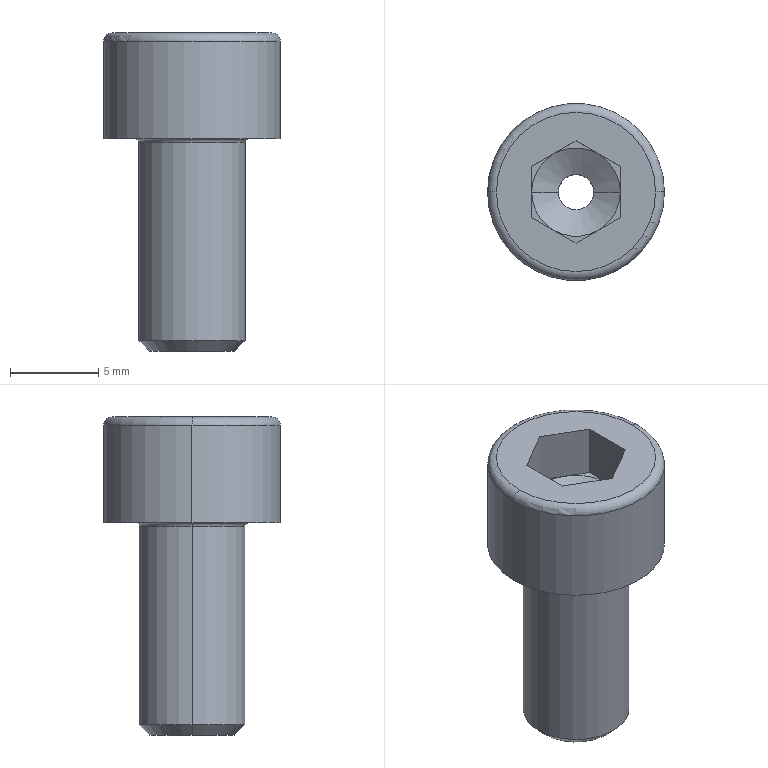Part | SolidWorks | features Fillet 2, ICE 2, Chamfer 1, Revolution 1 | 1 solid | 29 faces | box 10 x 10 x 18 mm | volume 687.683 mm3 | plane 15 | cylinder 6 | torus 4 | cone 4 | commonest cylinder face diameters 2 x2 6 x2 10 x2
STEP:
#1=CARTESIAN_POINT('',(-3.2,0.,0.));
#2=VERTEX_POINT('',#1);
#3=CARTESIAN_POINT('',(3.2,0.,0.));
#4=VERTEX_POINT('',#3);
#5=CARTESIAN_POINT('',(0.,0.,0.));
#6=DIRECTION('',(0.,0.,1.));
#7=DIRECTION('',(1.,0.,0.));
#8=AXIS2_PLACEMENT_3D('',#5,#6,#7);
#9=CIRCLE('',#8,3.2);
#10=EDGE_CURVE('',#2,#4,#9,.T.);
#11=ORIENTED_EDGE('',*,*,#10,.F.);
#12=CARTESIAN_POINT('',(-3.,0.,-0.2));
#13=VERTEX_POINT('',#12);
#14=CARTESIAN_POINT('',(-3.2,0.,-0.2));
#15=DIRECTION('',(0.,1.,0.));
#16=DIRECTION('',(-1.,0.,0.));
#17=AXIS2_PLACEMENT_3D('',#14,#15,#16);
#18=CIRCLE('',#17,0.2);
#19=EDGE_CURVE('',#2,#13,#18,.T.);
#20=ORIENTED_EDGE('',*,*,#19,.T.);
#21=CARTESIAN_POINT('',(3.,0.,-0.2));
#22=VERTEX_POINT('',#21);
#23=CARTESIAN_POINT('',(0.,0.,-0.2));
#24=DIRECTION('',(0.,0.,-1.));
#25=DIRECTION('',(1.,0.,0.));
#26=AXIS2_PLACEMENT_3D('',#23,#24,#25);
#27=CIRCLE('',#26,3.);
#28=EDGE_CURVE('',#22,#13,#27,.T.);
#29=ORIENTED_EDGE('',*,*,#28,.F.);
#30=CARTESIAN_POINT('',(3.2,0.,-0.2));
#31=DIRECTION('',(0.,-1.,0.));
#32=DIRECTION('',(0.,0.,-1.));
#33=AXIS2_PLACEMENT_3D('',#30,#31,#32);
#34=CIRCLE('',#33,0.2);
#35=EDGE_CURVE('',#4,#22,#34,.T.);
#36=ORIENTED_EDGE('',*,*,#35,.F.);
#37=EDGE_LOOP('',(#11,#20,#29,#36));
#38=FACE_OUTER_BOUND('',#37,.T.);
#39=CARTESIAN_POINT('',(0.,0.,-0.2));
#40=DIRECTION('',(0.,0.,1.));
#41=DIRECTION('',(1.,0.,0.));
#42=AXIS2_PLACEMENT_3D('',#39,#40,#41);
#43=TOROIDAL_SURFACE('',#42,3.2,0.2);
#44=ADVANCED_FACE('',(#38),#43,.F.);
#45=CARTESIAN_POINT('',(-1.,0.,2.134));
#46=VERTEX_POINT('',#45);
#47=CARTESIAN_POINT('',(1.,0.,2.134));
#48=VERTEX_POINT('',#47);
#49=CARTESIAN_POINT('',(0.,0.,2.134));
#50=DIRECTION('',(0.,0.,1.));
#51=DIRECTION('',(1.,0.,0.));
#52=AXIS2_PLACEMENT_3D('',#49,#50,#51);
#53=CIRCLE('',#52,1.);
#54=EDGE_CURVE('',#46,#48,#53,.T.);
#55=ORIENTED_EDGE('',*,*,#54,.F.);
#56=CARTESIAN_POINT('',(-2.5,0.,3.));
#57=VERTEX_POINT('',#56);
#58=CARTESIAN_POINT('',(-2.5,0.,3.));
#59=DIRECTION('',(-0.866,0.,0.5));
#60=VECTOR('',#59,1000.);
#61=LINE('',#58,#60);
#62=EDGE_CURVE('',#46,#57,#61,.T.);
#63=ORIENTED_EDGE('',*,*,#62,.T.);
#64=CARTESIAN_POINT('',(-1.25,-2.165,3.));
#65=VERTEX_POINT('',#64);
#66=CARTESIAN_POINT('',(0.,0.,3.));
#67=DIRECTION('',(0.,0.,1.));
#68=DIRECTION('',(1.,0.,0.));
#69=AXIS2_PLACEMENT_3D('',#66,#67,#68);
#70=CIRCLE('',#69,2.5);
#71=EDGE_CURVE('',#57,#65,#70,.T.);
#72=ORIENTED_EDGE('',*,*,#71,.T.);
#73=CARTESIAN_POINT('',(1.25,-2.165,3.));
#74=VERTEX_POINT('',#73);
#75=CARTESIAN_POINT('',(0.,0.,3.));
#76=DIRECTION('',(0.,0.,1.));
#77=DIRECTION('',(1.,0.,0.));
#78=AXIS2_PLACEMENT_3D('',#75,#76,#77);
#79=CIRCLE('',#78,2.5);
#80=EDGE_CURVE('',#65,#74,#79,.T.);
#81=ORIENTED_EDGE('',*,*,#80,.T.);
#82=CARTESIAN_POINT('',(2.5,0.,3.));
#83=VERTEX_POINT('',#82);
#84=CARTESIAN_POINT('',(0.,0.,3.));
#85=DIRECTION('',(0.,0.,1.));
#86=DIRECTION('',(1.,0.,0.));
#87=AXIS2_PLACEMENT_3D('',#84,#85,#86);
#88=CIRCLE('',#87,2.5);
#89=EDGE_CURVE('',#74,#83,#88,.T.);
#90=ORIENTED_EDGE('',*,*,#89,.T.);
#91=CARTESIAN_POINT('',(2.5,0.,3.));
#92=DIRECTION('',(0.866,0.,0.5));
#93=VECTOR('',#92,1000.);
#94=LINE('',#91,#93);
#95=EDGE_CURVE('',#48,#83,#94,.T.);
#96=ORIENTED_EDGE('',*,*,#95,.F.);
#97=EDGE_LOOP('',(#55,#63,#72,#81,#90,#96));
#98=FACE_OUTER_BOUND('',#97,.T.);
#99=CARTESIAN_POINT('',(0.,0.,3.));
#100=DIRECTION('',(0.,0.,1.));
#101=DIRECTION('',(1.,0.,0.));
#102=AXIS2_PLACEMENT_3D('',#99,#100,#101);
#103=CONICAL_SURFACE('',#102,2.5,1.047);
#104=ADVANCED_FACE('',(#98),#103,.F.);
#105=CARTESIAN_POINT('',(-2.4,0.,-12.));
#106=VERTEX_POINT('',#105);
#107=CARTESIAN_POINT('',(2.4,0.,-12.));
#108=VERTEX_POINT('',#107);
#109=CARTESIAN_POINT('',(0.,0.,-12.));
#110=DIRECTION('',(0.,0.,-1.));
#111=DIRECTION('',(1.,0.,0.));
#112=AXIS2_PLACEMENT_3D('',#109,#110,#111);
#113=CIRCLE('',#112,2.4);
#114=EDGE_CURVE('',#106,#108,#113,.T.);
#115=ORIENTED_EDGE('',*,*,#114,.F.);
#116=CARTESIAN_POINT('',(-3.,0.,-11.4));
#117=VERTEX_POINT('',#116);
#118=CARTESIAN_POINT('',(-3.,0.,-11.4));
#119=DIRECTION('',(-0.7071,0.,0.7071));
#120=VECTOR('',#119,1000.);
#121=LINE('',#118,#120);
#122=EDGE_CURVE('',#106,#117,#121,.T.);
#123=ORIENTED_EDGE('',*,*,#122,.T.);
#124=CARTESIAN_POINT('',(3.,0.,-11.4));
#125=VERTEX_POINT('',#124);
#126=CARTESIAN_POINT('',(0.,0.,-11.4));
#127=DIRECTION('',(0.,0.,1.));
#128=DIRECTION('',(1.,0.,0.));
#129=AXIS2_PLACEMENT_3D('',#126,#127,#128);
#130=CIRCLE('',#129,3.);
#131=EDGE_CURVE('',#125,#117,#130,.T.);
#132=ORIENTED_EDGE('',*,*,#131,.F.);
#133=CARTESIAN_POINT('',(3.,0.,-11.4));
#134=DIRECTION('',(0.7071,0.,0.7071));
#135=VECTOR('',#134,1000.);
#136=LINE('',#133,#135);
#137=EDGE_CURVE('',#108,#125,#136,.T.);
#138=ORIENTED_EDGE('',*,*,#137,.F.);
#139=EDGE_LOOP('',(#115,#123,#132,#138));
#140=FACE_OUTER_BOUND('',#139,.T.);
#141=CARTESIAN_POINT('',(0.,0.,-11.4));
#142=DIRECTION('',(0.,0.,1.));
#143=DIRECTION('',(1.,0.,0.));
#144=AXIS2_PLACEMENT_3D('',#141,#142,#143);
#145=CONICAL_SURFACE('',#144,3.,0.7854);
#146=ADVANCED_FACE('',(#140),#145,.T.);
#147=CARTESIAN_POINT('',(4.5,0.,6.));
#148=VERTEX_POINT('',#147);
#149=CARTESIAN_POINT('',(-4.5,0.,6.));
#150=VERTEX_POINT('',#149);
#151=CARTESIAN_POINT('',(0.,0.,6.));
#152=DIRECTION('',(0.,0.,1.));
#153=DIRECTION('',(-1.,0.,0.));
#154=AXIS2_PLACEMENT_3D('',#151,#152,#153);
#155=CIRCLE('',#154,4.5);
#156=EDGE_CURVE('',#148,#150,#155,.T.);
#157=ORIENTED_EDGE('',*,*,#156,.F.);
#158=CARTESIAN_POINT('',(5.,0.,5.5));
#159=VERTEX_POINT('',#158);
#160=CARTESIAN_POINT('',(4.5,0.,5.5));
#161=DIRECTION('',(0.,1.,0.));
#162=DIRECTION('',(-1.,0.,0.));
#163=AXIS2_PLACEMENT_3D('',#160,#161,#162);
#164=CIRCLE('',#163,0.5);
#165=EDGE_CURVE('',#148,#159,#164,.T.);
#166=ORIENTED_EDGE('',*,*,#165,.T.);
#167=CARTESIAN_POINT('',(-5.,0.,5.5));
#168=VERTEX_POINT('',#167);
#169=CARTESIAN_POINT('',(0.,0.,5.5));
#170=DIRECTION('',(0.,0.,-1.));
#171=DIRECTION('',(-1.,0.,0.));
#172=AXIS2_PLACEMENT_3D('',#169,#170,#171);
#173=CIRCLE('',#172,5.);
#174=EDGE_CURVE('',#168,#159,#173,.T.);
#175=ORIENTED_EDGE('',*,*,#174,.F.);
#176=CARTESIAN_POINT('',(-4.5,0.,5.5));
#177=DIRECTION('',(0.,-1.,0.));
#178=DIRECTION('',(0.,0.,-1.));
#179=AXIS2_PLACEMENT_3D('',#176,#177,#178);
#180=CIRCLE('',#179,0.5);
#181=EDGE_CURVE('',#150,#168,#180,.T.);
#182=ORIENTED_EDGE('',*,*,#181,.F.);
#183=EDGE_LOOP('',(#157,#166,#175,#182));
#184=FACE_OUTER_BOUND('',#183,.T.);
#185=CARTESIAN_POINT('',(0.,0.,5.5));
#186=DIRECTION('',(0.,0.,-1.));
#187=DIRECTION('',(-1.,0.,0.));
#188=AXIS2_PLACEMENT_3D('',#185,#186,#187);
#189=TOROIDAL_SURFACE('',#188,4.5,0.5);
#190=ADVANCED_FACE('',(#184),#189,.T.);
#191=ORIENTED_EDGE('',*,*,#131,.T.);
#192=CARTESIAN_POINT('',(-3.,0.,6.));
#193=DIRECTION('',(0.,0.,1.));
#194=VECTOR('',#193,1000.);
#195=LINE('',#192,#194);
#196=EDGE_CURVE('',#117,#13,#195,.T.);
#197=ORIENTED_EDGE('',*,*,#196,.T.);
#198=CARTESIAN_POINT('',(0.,0.,-0.2));
#199=DIRECTION('',(0.,0.,-1.));
#200=DIRECTION('',(1.,0.,0.));
#201=AXIS2_PLACEMENT_3D('',#198,#199,#200);
#202=CIRCLE('',#201,3.);
#203=EDGE_CURVE('',#13,#22,#202,.T.);
#204=ORIENTED_EDGE('',*,*,#203,.T.);
#205=CARTESIAN_POINT('',(3.,0.,6.));
#206=DIRECTION('',(0.,0.,1.));
#207=VECTOR('',#206,1000.);
#208=LINE('',#205,#207);
#209=EDGE_CURVE('',#125,#22,#208,.T.);
#210=ORIENTED_EDGE('',*,*,#209,.F.);
#211=EDGE_LOOP('',(#191,#197,#204,#210));
#212=FACE_OUTER_BOUND('',#211,.T.);
#213=CARTESIAN_POINT('',(0.,0.,6.));
#214=DIRECTION('',(0.,0.,1.));
#215=DIRECTION('',(1.,0.,0.));
#216=AXIS2_PLACEMENT_3D('',#213,#214,#215);
#217=CYLINDRICAL_SURFACE('',#216,3.);
#218=ADVANCED_FACE('',(#212),#217,.T.);
#219=CARTESIAN_POINT('',(5.,0.,0.));
#220=VERTEX_POINT('',#219);
#221=CARTESIAN_POINT('',(-5.,0.,0.));
#222=VERTEX_POINT('',#221);
#223=CARTESIAN_POINT('',(0.,0.,0.));
#224=DIRECTION('',(0.,0.,1.));
#225=DIRECTION('',(1.,0.,0.));
#226=AXIS2_PLACEMENT_3D('',#223,#224,#225);
#227=CIRCLE('',#226,5.);
#228=EDGE_CURVE('',#220,#222,#227,.T.);
#229=ORIENTED_EDGE('',*,*,#228,.T.);
#230=CARTESIAN_POINT('',(-5.,0.,6.));
#231=DIRECTION('',(0.,0.,1.));
#232=VECTOR('',#231,1000.);
#233=LINE('',#230,#232);
#234=EDGE_CURVE('',#222,#168,#233,.T.);
#235=ORIENTED_EDGE('',*,*,#234,.T.);
#236=ORIENTED_EDGE('',*,*,#174,.T.);
#237=CARTESIAN_POINT('',(5.,0.,6.));
#238=DIRECTION('',(0.,0.,1.));
#239=VECTOR('',#238,1000.);
#240=LINE('',#237,#239);
#241=EDGE_CURVE('',#220,#159,#240,.T.);
#242=ORIENTED_EDGE('',*,*,#241,.F.);
#243=EDGE_LOOP('',(#229,#235,#236,#242));
#244=FACE_OUTER_BOUND('',#243,.T.);
#245=CARTESIAN_POINT('',(0.,0.,6.));
#246=DIRECTION('',(0.,0.,1.));
#247=DIRECTION('',(1.,0.,0.));
#248=AXIS2_PLACEMENT_3D('',#245,#246,#247);
#249=CYLINDRICAL_SURFACE('',#248,5.);
#250=ADVANCED_FACE('',(#244),#249,.T.);
#251=CARTESIAN_POINT('',(-1.,0.,-12.));
#252=VERTEX_POINT('',#251);
#253=CARTESIAN_POINT('',(1.,0.,-12.));
#254=VERTEX_POINT('',#253);
#255=CARTESIAN_POINT('',(0.,0.,-12.));
#256=DIRECTION('',(0.,0.,1.));
#257=DIRECTION('',(1.,0.,0.));
#258=AXIS2_PLACEMENT_3D('',#255,#256,#257);
#259=CIRCLE('',#258,1.);
#260=EDGE_CURVE('',#252,#254,#259,.T.);
#261=ORIENTED_EDGE('',*,*,#260,.F.);
#262=CARTESIAN_POINT('',(-1.,0.,6.));
#263=DIRECTION('',(0.,0.,1.));
#264=VECTOR('',#263,1000.);
#265=LINE('',#262,#264);
#266=EDGE_CURVE('',#252,#46,#265,.T.);
#267=ORIENTED_EDGE('',*,*,#266,.T.);
#268=ORIENTED_EDGE('',*,*,#54,.T.);
#269=CARTESIAN_POINT('',(1.,0.,6.));
#270=DIRECTION('',(0.,0.,1.));
#271=VECTOR('',#270,1000.);
#272=LINE('',#269,#271);
#273=EDGE_CURVE('',#254,#48,#272,.T.);
#274=ORIENTED_EDGE('',*,*,#273,.F.);
#275=EDGE_LOOP('',(#261,#267,#268,#274));
#276=FACE_OUTER_BOUND('',#275,.T.);
#277=CARTESIAN_POINT('',(0.,0.,6.));
#278=DIRECTION('',(0.,0.,1.));
#279=DIRECTION('',(1.,0.,0.));
#280=AXIS2_PLACEMENT_3D('',#277,#278,#279);
#281=CYLINDRICAL_SURFACE('',#280,1.);
#282=ADVANCED_FACE('',(#276),#281,.F.);
#283=CARTESIAN_POINT('',(1.25,2.165,3.));
#284=VERTEX_POINT('',#283);
#285=CARTESIAN_POINT('',(0.,0.,3.));
#286=DIRECTION('',(0.,0.,1.));
#287=DIRECTION('',(1.,0.,0.));
#288=AXIS2_PLACEMENT_3D('',#285,#286,#287);
#289=CIRCLE('',#288,2.5);
#290=EDGE_CURVE('',#83,#284,#289,.T.);
#291=ORIENTED_EDGE('',*,*,#290,.F.);
#292=CARTESIAN_POINT('',(2.5,1.443,3.));
#293=VERTEX_POINT('',#292);
#294=CARTESIAN_POINT('',(2.5,-1.443,3.));
#295=DIRECTION('',(0.,1.,0.));
#296=VECTOR('',#295,1000.);
#297=LINE('',#294,#296);
#298=EDGE_CURVE('',#83,#293,#297,.T.);
#299=ORIENTED_EDGE('',*,*,#298,.T.);
#300=CARTESIAN_POINT('',(2.5,1.443,3.));
#301=DIRECTION('',(-0.866,0.5,0.));
#302=VECTOR('',#301,1000.);
#303=LINE('',#300,#302);
#304=EDGE_CURVE('',#293,#284,#303,.T.);
#305=ORIENTED_EDGE('',*,*,#304,.T.);
#306=EDGE_LOOP('',(#291,#299,#305));
#307=FACE_OUTER_BOUND('',#306,.T.);
#308=CARTESIAN_POINT('',(0.,2.887,3.));
#309=DIRECTION('',(0.,0.,1.));
#310=DIRECTION('',(1.,0.,0.));
#311=AXIS2_PLACEMENT_3D('',#308,#309,#310);
#312=PLANE('',#311);
#313=ADVANCED_FACE('',(#307),#312,.T.);
#314=CARTESIAN_POINT('',(-1.25,2.165,3.));
#315=VERTEX_POINT('',#314);
#316=CARTESIAN_POINT('',(0.,0.,3.));
#317=DIRECTION('',(0.,0.,1.));
#318=DIRECTION('',(1.,0.,0.));
#319=AXIS2_PLACEMENT_3D('',#316,#317,#318);
#320=CIRCLE('',#319,2.5);
#321=EDGE_CURVE('',#284,#315,#320,.T.);
#322=ORIENTED_EDGE('',*,*,#321,.F.);
#323=CARTESIAN_POINT('',(0.,2.887,3.));
#324=VERTEX_POINT('',#323);
#325=CARTESIAN_POINT('',(2.5,1.443,3.));
#326=DIRECTION('',(-0.866,0.5,0.));
#327=VECTOR('',#326,1000.);
#328=LINE('',#325,#327);
#329=EDGE_CURVE('',#284,#324,#328,.T.);
#330=ORIENTED_EDGE('',*,*,#329,.T.);
#331=CARTESIAN_POINT('',(0.,2.887,3.));
#332=DIRECTION('',(-0.866,-0.5,0.));
#333=VECTOR('',#332,1000.);
#334=LINE('',#331,#333);
#335=EDGE_CURVE('',#324,#315,#334,.T.);
#336=ORIENTED_EDGE('',*,*,#335,.T.);
#337=EDGE_LOOP('',(#322,#330,#336));
#338=FACE_OUTER_BOUND('',#337,.T.);
#339=CARTESIAN_POINT('',(0.,2.887,3.));
#340=DIRECTION('',(0.,0.,1.));
#341=DIRECTION('',(1.,0.,0.));
#342=AXIS2_PLACEMENT_3D('',#339,#340,#341);
#343=PLANE('',#342);
#344=ADVANCED_FACE('',(#338),#343,.T.);
#345=CARTESIAN_POINT('',(0.,0.,3.));
#346=DIRECTION('',(0.,0.,1.));
#347=DIRECTION('',(1.,0.,0.));
#348=AXIS2_PLACEMENT_3D('',#345,#346,#347);
#349=CIRCLE('',#348,2.5);
#350=EDGE_CURVE('',#315,#57,#349,.T.);
#351=ORIENTED_EDGE('',*,*,#350,.F.);
#352=CARTESIAN_POINT('',(-2.5,1.443,3.));
#353=VERTEX_POINT('',#352);
#354=CARTESIAN_POINT('',(0.,2.887,3.));
#355=DIRECTION('',(-0.866,-0.5,0.));
#356=VECTOR('',#355,1000.);
#357=LINE('',#354,#356);
#358=EDGE_CURVE('',#315,#353,#357,.T.);
#359=ORIENTED_EDGE('',*,*,#358,.T.);
#360=CARTESIAN_POINT('',(-2.5,1.443,3.));
#361=DIRECTION('',(0.,-1.,0.));
#362=VECTOR('',#361,1000.);
#363=LINE('',#360,#362);
#364=EDGE_CURVE('',#353,#57,#363,.T.);
#365=ORIENTED_EDGE('',*,*,#364,.T.);
#366=EDGE_LOOP('',(#351,#359,#365));
#367=FACE_OUTER_BOUND('',#366,.T.);
#368=CARTESIAN_POINT('',(0.,2.887,3.));
#369=DIRECTION('',(0.,0.,1.));
#370=DIRECTION('',(1.,0.,0.));
#371=AXIS2_PLACEMENT_3D('',#368,#369,#370);
#372=PLANE('',#371);
#373=ADVANCED_FACE('',(#367),#372,.T.);
#374=ORIENTED_EDGE('',*,*,#71,.F.);
#375=CARTESIAN_POINT('',(-2.5,-1.443,3.));
#376=VERTEX_POINT('',#375);
#377=CARTESIAN_POINT('',(-2.5,1.443,3.));
#378=DIRECTION('',(0.,-1.,0.));
#379=VECTOR('',#378,1000.);
#380=LINE('',#377,#379);
#381=EDGE_CURVE('',#57,#376,#380,.T.);
#382=ORIENTED_EDGE('',*,*,#381,.T.);
#383=CARTESIAN_POINT('',(-2.5,-1.443,3.));
#384=DIRECTION('',(0.866,-0.5,0.));
#385=VECTOR('',#384,1000.);
#386=LINE('',#383,#385);
#387=EDGE_CURVE('',#376,#65,#386,.T.);
#388=ORIENTED_EDGE('',*,*,#387,.T.);
#389=EDGE_LOOP('',(#374,#382,#388));
#390=FACE_OUTER_BOUND('',#389,.T.);
#391=CARTESIAN_POINT('',(0.,2.887,3.));
#392=DIRECTION('',(0.,0.,1.));
#393=DIRECTION('',(1.,0.,0.));
#394=AXIS2_PLACEMENT_3D('',#391,#392,#393);
#395=PLANE('',#394);
#396=ADVANCED_FACE('',(#390),#395,.T.);
#397=ORIENTED_EDGE('',*,*,#80,.F.);
#398=CARTESIAN_POINT('',(0.,-2.887,3.));
#399=VERTEX_POINT('',#398);
#400=CARTESIAN_POINT('',(-2.5,-1.443,3.));
#401=DIRECTION('',(0.866,-0.5,0.));
#402=VECTOR('',#401,1000.);
#403=LINE('',#400,#402);
#404=EDGE_CURVE('',#65,#399,#403,.T.);
#405=ORIENTED_EDGE('',*,*,#404,.T.);
#406=CARTESIAN_POINT('',(0.,-2.887,3.));
#407=DIRECTION('',(0.866,0.5,0.));
#408=VECTOR('',#407,1000.);
#409=LINE('',#406,#408);
#410=EDGE_CURVE('',#399,#74,#409,.T.);
#411=ORIENTED_EDGE('',*,*,#410,.T.);
#412=EDGE_LOOP('',(#397,#405,#411));
#413=FACE_OUTER_BOUND('',#412,.T.);
#414=CARTESIAN_POINT('',(0.,2.887,3.));
#415=DIRECTION('',(0.,0.,1.));
#416=DIRECTION('',(1.,0.,0.));
#417=AXIS2_PLACEMENT_3D('',#414,#415,#416);
#418=PLANE('',#417);
#419=ADVANCED_FACE('',(#413),#418,.T.);
#420=ORIENTED_EDGE('',*,*,#266,.F.);
#421=CARTESIAN_POINT('',(0.,0.,-12.));
#422=DIRECTION('',(0.,0.,1.));
#423=DIRECTION('',(1.,0.,0.));
#424=AXIS2_PLACEMENT_3D('',#421,#422,#423);
#425=CIRCLE('',#424,1.);
#426=EDGE_CURVE('',#254,#252,#425,.T.);
#427=ORIENTED_EDGE('',*,*,#426,.F.);
#428=ORIENTED_EDGE('',*,*,#273,.T.);
#429=CARTESIAN_POINT('',(0.,0.,2.134));
#430=DIRECTION('',(0.,0.,1.));
#431=DIRECTION('',(1.,0.,0.));
#432=AXIS2_PLACEMENT_3D('',#429,#430,#431);
#433=CIRCLE('',#432,1.);
#434=EDGE_CURVE('',#48,#46,#433,.T.);
#435=ORIENTED_EDGE('',*,*,#434,.T.);
#436=EDGE_LOOP('',(#420,#427,#428,#435));
#437=FACE_OUTER_BOUND('',#436,.T.);
#438=CARTESIAN_POINT('',(0.,0.,6.));
#439=DIRECTION('',(0.,0.,1.));
#440=DIRECTION('',(1.,0.,0.));
#441=AXIS2_PLACEMENT_3D('',#438,#439,#440);
#442=CYLINDRICAL_SURFACE('',#441,1.);
#443=ADVANCED_FACE('',(#437),#442,.F.);
#444=ORIENTED_EDGE('',*,*,#234,.F.);
#445=CARTESIAN_POINT('',(0.,0.,0.));
#446=DIRECTION('',(0.,0.,1.));
#447=DIRECTION('',(1.,0.,0.));
#448=AXIS2_PLACEMENT_3D('',#445,#446,#447);
#449=CIRCLE('',#448,5.);
#450=EDGE_CURVE('',#222,#220,#449,.T.);
#451=ORIENTED_EDGE('',*,*,#450,.T.);
#452=ORIENTED_EDGE('',*,*,#241,.T.);
#453=CARTESIAN_POINT('',(0.,0.,5.5));
#454=DIRECTION('',(0.,0.,-1.));
#455=DIRECTION('',(-1.,0.,0.));
#456=AXIS2_PLACEMENT_3D('',#453,#454,#455);
#457=CIRCLE('',#456,5.);
#458=EDGE_CURVE('',#159,#168,#457,.T.);
#459=ORIENTED_EDGE('',*,*,#458,.T.);
#460=EDGE_LOOP('',(#444,#451,#452,#459));
#461=FACE_OUTER_BOUND('',#460,.T.);
#462=CARTESIAN_POINT('',(0.,0.,6.));
#463=DIRECTION('',(0.,0.,1.));
#464=DIRECTION('',(1.,0.,0.));
#465=AXIS2_PLACEMENT_3D('',#462,#463,#464);
#466=CYLINDRICAL_SURFACE('',#465,5.);
#467=ADVANCED_FACE('',(#461),#466,.T.);
#468=CARTESIAN_POINT('',(0.,0.,0.));
#469=DIRECTION('',(0.,0.,1.));
#470=DIRECTION('',(1.,0.,0.));
#471=AXIS2_PLACEMENT_3D('',#468,#469,#470);
#472=CIRCLE('',#471,3.2);
#473=EDGE_CURVE('',#4,#2,#472,.T.);
#474=ORIENTED_EDGE('',*,*,#473,.T.);
#475=ORIENTED_EDGE('',*,*,#10,.T.);
#476=EDGE_LOOP('',(#474,#475));
#477=FACE_BOUND('',#476,.T.);
#478=ORIENTED_EDGE('',*,*,#228,.F.);
#479=ORIENTED_EDGE('',*,*,#450,.F.);
#480=EDGE_LOOP('',(#478,#479));
#481=FACE_OUTER_BOUND('',#480,.T.);
#482=CARTESIAN_POINT('',(0.,5.,0.));
#483=DIRECTION('',(0.,0.,1.));
#484=DIRECTION('',(1.,0.,0.));
#485=AXIS2_PLACEMENT_3D('',#482,#483,#484);
#486=PLANE('',#485);
#487=ADVANCED_FACE('',(#477,#481),#486,.F.);
#488=ORIENTED_EDGE('',*,*,#196,.F.);
#489=CARTESIAN_POINT('',(0.,0.,-11.4));
#490=DIRECTION('',(0.,0.,1.));
#491=DIRECTION('',(1.,0.,0.));
#492=AXIS2_PLACEMENT_3D('',#489,#490,#491);
#493=CIRCLE('',#492,3.);
#494=EDGE_CURVE('',#117,#125,#493,.T.);
#495=ORIENTED_EDGE('',*,*,#494,.T.);
#496=ORIENTED_EDGE('',*,*,#209,.T.);
#497=ORIENTED_EDGE('',*,*,#28,.T.);
#498=EDGE_LOOP('',(#488,#495,#496,#497));
#499=FACE_OUTER_BOUND('',#498,.T.);
#500=CARTESIAN_POINT('',(0.,0.,6.));
#501=DIRECTION('',(0.,0.,1.));
#502=DIRECTION('',(1.,0.,0.));
#503=AXIS2_PLACEMENT_3D('',#500,#501,#502);
#504=CYLINDRICAL_SURFACE('',#503,3.);
#505=ADVANCED_FACE('',(#499),#504,.T.);
#506=CARTESIAN_POINT('',(0.,0.,-12.));
#507=DIRECTION('',(0.,0.,-1.));
#508=DIRECTION('',(1.,0.,0.));
#509=AXIS2_PLACEMENT_3D('',#506,#507,#508);
#510=CIRCLE('',#509,2.4);
#511=EDGE_CURVE('',#108,#106,#510,.T.);
#512=ORIENTED_EDGE('',*,*,#511,.T.);
#513=ORIENTED_EDGE('',*,*,#114,.T.);
#514=EDGE_LOOP('',(#512,#513));
#515=FACE_OUTER_BOUND('',#514,.T.);
#516=ORIENTED_EDGE('',*,*,#426,.T.);
#517=ORIENTED_EDGE('',*,*,#260,.T.);
#518=EDGE_LOOP('',(#516,#517));
#519=FACE_BOUND('',#518,.T.);
#520=CARTESIAN_POINT('',(0.,3.,-12.));
#521=DIRECTION('',(0.,0.,1.));
#522=DIRECTION('',(1.,0.,0.));
#523=AXIS2_PLACEMENT_3D('',#520,#521,#522);
#524=PLANE('',#523);
#525=ADVANCED_FACE('',(#515,#519),#524,.F.);
#526=CARTESIAN_POINT('',(0.,0.,6.));
#527=DIRECTION('',(0.,0.,1.));
#528=DIRECTION('',(-1.,0.,0.));
#529=AXIS2_PLACEMENT_3D('',#526,#527,#528);
#530=CIRCLE('',#529,4.5);
#531=EDGE_CURVE('',#150,#148,#530,.T.);
#532=ORIENTED_EDGE('',*,*,#531,.T.);
#533=ORIENTED_EDGE('',*,*,#156,.T.);
#534=EDGE_LOOP('',(#532,#533));
#535=FACE_OUTER_BOUND('',#534,.T.);
#536=CARTESIAN_POINT('',(0.,2.887,6.));
#537=VERTEX_POINT('',#536);
#538=CARTESIAN_POINT('',(-2.5,1.443,6.));
#539=VERTEX_POINT('',#538);
#540=CARTESIAN_POINT('',(0.,2.887,6.));
#541=DIRECTION('',(-0.866,-0.5,0.));
#542=VECTOR('',#541,1000.);
#543=LINE('',#540,#542);
#544=EDGE_CURVE('',#537,#539,#543,.T.);
#545=ORIENTED_EDGE('',*,*,#544,.F.);
#546=CARTESIAN_POINT('',(2.5,1.443,6.));
#547=VERTEX_POINT('',#546);
#548=CARTESIAN_POINT('',(2.5,1.443,6.));
#549=DIRECTION('',(-0.866,0.5,0.));
#550=VECTOR('',#549,1000.);
#551=LINE('',#548,#550);
#552=EDGE_CURVE('',#547,#537,#551,.T.);
#553=ORIENTED_EDGE('',*,*,#552,.F.);
#554=CARTESIAN_POINT('',(2.5,-1.443,6.));
#555=VERTEX_POINT('',#554);
#556=CARTESIAN_POINT('',(2.5,-1.443,6.));
#557=DIRECTION('',(0.,1.,0.));
#558=VECTOR('',#557,1000.);
#559=LINE('',#556,#558);
#560=EDGE_CURVE('',#555,#547,#559,.T.);
#561=ORIENTED_EDGE('',*,*,#560,.F.);
#562=CARTESIAN_POINT('',(0.,-2.887,6.));
#563=VERTEX_POINT('',#562);
#564=CARTESIAN_POINT('',(0.,-2.887,6.));
#565=DIRECTION('',(0.866,0.5,0.));
#566=VECTOR('',#565,1000.);
#567=LINE('',#564,#566);
#568=EDGE_CURVE('',#563,#555,#567,.T.);
#569=ORIENTED_EDGE('',*,*,#568,.F.);
#570=CARTESIAN_POINT('',(-2.5,-1.443,6.));
#571=VERTEX_POINT('',#570);
#572=CARTESIAN_POINT('',(-2.5,-1.443,6.));
#573=DIRECTION('',(0.866,-0.5,0.));
#574=VECTOR('',#573,1000.);
#575=LINE('',#572,#574);
#576=EDGE_CURVE('',#571,#563,#575,.T.);
#577=ORIENTED_EDGE('',*,*,#576,.F.);
#578=CARTESIAN_POINT('',(-2.5,1.443,6.));
#579=DIRECTION('',(0.,-1.,0.));
#580=VECTOR('',#579,1000.);
#581=LINE('',#578,#580);
#582=EDGE_CURVE('',#539,#571,#581,.T.);
#583=ORIENTED_EDGE('',*,*,#582,.F.);
#584=EDGE_LOOP('',(#545,#553,#561,#569,#577,#583));
#585=FACE_BOUND('',#584,.T.);
#586=CARTESIAN_POINT('',(0.,1.,6.));
#587=DIRECTION('',(0.,0.,-1.));
#588=DIRECTION('',(-1.,0.,0.));
#589=AXIS2_PLACEMENT_3D('',#586,#587,#588);
#590=PLANE('',#589);
#591=ADVANCED_FACE('',(#535,#585),#590,.F.);
#592=ORIENTED_EDGE('',*,*,#89,.F.);
#593=CARTESIAN_POINT('',(2.5,-1.443,3.));
#594=VERTEX_POINT('',#593);
#595=CARTESIAN_POINT('',(0.,-2.887,3.));
#596=DIRECTION('',(0.866,0.5,0.));
#597=VECTOR('',#596,1000.);
#598=LINE('',#595,#597);
#599=EDGE_CURVE('',#74,#594,#598,.T.);
#600=ORIENTED_EDGE('',*,*,#599,.T.);
#601=CARTESIAN_POINT('',(2.5,-1.443,3.));
#602=DIRECTION('',(0.,1.,0.));
#603=VECTOR('',#602,1000.);
#604=LINE('',#601,#603);
#605=EDGE_CURVE('',#594,#83,#604,.T.);
#606=ORIENTED_EDGE('',*,*,#605,.T.);
#607=EDGE_LOOP('',(#592,#600,#606));
#608=FACE_OUTER_BOUND('',#607,.T.);
#609=CARTESIAN_POINT('',(0.,2.887,3.));
#610=DIRECTION('',(0.,0.,1.));
#611=DIRECTION('',(1.,0.,0.));
#612=AXIS2_PLACEMENT_3D('',#609,#610,#611);
#613=PLANE('',#612);
#614=ADVANCED_FACE('',(#608),#613,.T.);
#615=ORIENTED_EDGE('',*,*,#552,.T.);
#616=CARTESIAN_POINT('',(0.,2.887,3.));
#617=DIRECTION('',(0.,0.,1.));
#618=VECTOR('',#617,1000.);
#619=LINE('',#616,#618);
#620=EDGE_CURVE('',#324,#537,#619,.T.);
#621=ORIENTED_EDGE('',*,*,#620,.F.);
#622=ORIENTED_EDGE('',*,*,#329,.F.);
#623=ORIENTED_EDGE('',*,*,#304,.F.);
#624=CARTESIAN_POINT('',(2.5,1.443,3.));
#625=DIRECTION('',(0.,0.,1.));
#626=VECTOR('',#625,1000.);
#627=LINE('',#624,#626);
#628=EDGE_CURVE('',#293,#547,#627,.T.);
#629=ORIENTED_EDGE('',*,*,#628,.T.);
#630=EDGE_LOOP('',(#615,#621,#622,#623,#629));
#631=FACE_OUTER_BOUND('',#630,.T.);
#632=CARTESIAN_POINT('',(2.5,1.443,3.));
#633=DIRECTION('',(0.5,0.866,0.));
#634=DIRECTION('',(-0.866,0.5,0.));
#635=AXIS2_PLACEMENT_3D('',#632,#633,#634);
#636=PLANE('',#635);
#637=ADVANCED_FACE('',(#631),#636,.F.);
#638=ORIENTED_EDGE('',*,*,#560,.T.);
#639=ORIENTED_EDGE('',*,*,#628,.F.);
#640=ORIENTED_EDGE('',*,*,#298,.F.);
#641=ORIENTED_EDGE('',*,*,#605,.F.);
#642=CARTESIAN_POINT('',(2.5,-1.443,3.));
#643=DIRECTION('',(0.,0.,1.));
#644=VECTOR('',#643,1000.);
#645=LINE('',#642,#644);
#646=EDGE_CURVE('',#594,#555,#645,.T.);
#647=ORIENTED_EDGE('',*,*,#646,.T.);
#648=EDGE_LOOP('',(#638,#639,#640,#641,#647));
#649=FACE_OUTER_BOUND('',#648,.T.);
#650=CARTESIAN_POINT('',(2.5,-1.443,3.));
#651=DIRECTION('',(1.,0.,0.));
#652=DIRECTION('',(0.,0.,-1.));
#653=AXIS2_PLACEMENT_3D('',#650,#651,#652);
#654=PLANE('',#653);
#655=ADVANCED_FACE('',(#649),#654,.F.);
#656=ORIENTED_EDGE('',*,*,#568,.T.);
#657=ORIENTED_EDGE('',*,*,#646,.F.);
#658=ORIENTED_EDGE('',*,*,#599,.F.);
#659=ORIENTED_EDGE('',*,*,#410,.F.);
#660=CARTESIAN_POINT('',(0.,-2.887,3.));
#661=DIRECTION('',(0.,0.,1.));
#662=VECTOR('',#661,1000.);
#663=LINE('',#660,#662);
#664=EDGE_CURVE('',#399,#563,#663,.T.);
#665=ORIENTED_EDGE('',*,*,#664,.T.);
#666=EDGE_LOOP('',(#656,#657,#658,#659,#665));
#667=FACE_OUTER_BOUND('',#666,.T.);
#668=CARTESIAN_POINT('',(0.,-2.887,3.));
#669=DIRECTION('',(0.5,-0.866,0.));
#670=DIRECTION('',(0.866,0.5,0.));
#671=AXIS2_PLACEMENT_3D('',#668,#669,#670);
#672=PLANE('',#671);
#673=ADVANCED_FACE('',(#667),#672,.F.);
#674=ORIENTED_EDGE('',*,*,#576,.T.);
#675=ORIENTED_EDGE('',*,*,#664,.F.);
#676=ORIENTED_EDGE('',*,*,#404,.F.);
#677=ORIENTED_EDGE('',*,*,#387,.F.);
#678=CARTESIAN_POINT('',(-2.5,-1.443,3.));
#679=DIRECTION('',(0.,0.,1.));
#680=VECTOR('',#679,1000.);
#681=LINE('',#678,#680);
#682=EDGE_CURVE('',#376,#571,#681,.T.);
#683=ORIENTED_EDGE('',*,*,#682,.T.);
#684=EDGE_LOOP('',(#674,#675,#676,#677,#683));
#685=FACE_OUTER_BOUND('',#684,.T.);
#686=CARTESIAN_POINT('',(-2.5,-1.443,3.));
#687=DIRECTION('',(-0.5,-0.866,0.));
#688=DIRECTION('',(0.866,-0.5,0.));
#689=AXIS2_PLACEMENT_3D('',#686,#687,#688);
#690=PLANE('',#689);
#691=ADVANCED_FACE('',(#685),#690,.F.);
#692=ORIENTED_EDGE('',*,*,#582,.T.);
#693=ORIENTED_EDGE('',*,*,#682,.F.);
#694=ORIENTED_EDGE('',*,*,#381,.F.);
#695=ORIENTED_EDGE('',*,*,#364,.F.);
#696=CARTESIAN_POINT('',(-2.5,1.443,3.));
#697=DIRECTION('',(0.,0.,1.));
#698=VECTOR('',#697,1000.);
#699=LINE('',#696,#698);
#700=EDGE_CURVE('',#353,#539,#699,.T.);
#701=ORIENTED_EDGE('',*,*,#700,.T.);
#702=EDGE_LOOP('',(#692,#693,#694,#695,#701));
#703=FACE_OUTER_BOUND('',#702,.T.);
#704=CARTESIAN_POINT('',(-2.5,1.443,3.));
#705=DIRECTION('',(-1.,0.,0.));
#706=DIRECTION('',(0.,-1.,0.));
#707=AXIS2_PLACEMENT_3D('',#704,#705,#706);
#708=PLANE('',#707);
#709=ADVANCED_FACE('',(#703),#708,.F.);
#710=ORIENTED_EDGE('',*,*,#544,.T.);
#711=ORIENTED_EDGE('',*,*,#700,.F.);
#712=ORIENTED_EDGE('',*,*,#358,.F.);
#713=ORIENTED_EDGE('',*,*,#335,.F.);
#714=ORIENTED_EDGE('',*,*,#620,.T.);
#715=EDGE_LOOP('',(#710,#711,#712,#713,#714));
#716=FACE_OUTER_BOUND('',#715,.T.);
#717=CARTESIAN_POINT('',(0.,2.887,3.));
#718=DIRECTION('',(-0.5,0.866,0.));
#719=DIRECTION('',(-0.866,-0.5,0.));
#720=AXIS2_PLACEMENT_3D('',#717,#718,#719);
#721=PLANE('',#720);
#722=ADVANCED_FACE('',(#716),#721,.F.);
#723=ORIENTED_EDGE('',*,*,#165,.F.);
#724=ORIENTED_EDGE('',*,*,#531,.F.);
#725=ORIENTED_EDGE('',*,*,#181,.T.);
#726=ORIENTED_EDGE('',*,*,#458,.F.);
#727=EDGE_LOOP('',(#723,#724,#725,#726));
#728=FACE_OUTER_BOUND('',#727,.T.);
#729=CARTESIAN_POINT('',(0.,0.,5.5));
#730=DIRECTION('',(0.,0.,-1.));
#731=DIRECTION('',(-1.,0.,0.));
#732=AXIS2_PLACEMENT_3D('',#729,#730,#731);
#733=TOROIDAL_SURFACE('',#732,4.5,0.5);
#734=ADVANCED_FACE('',(#728),#733,.T.);
#735=ORIENTED_EDGE('',*,*,#122,.F.);
#736=ORIENTED_EDGE('',*,*,#511,.F.);
#737=ORIENTED_EDGE('',*,*,#137,.T.);
#738=ORIENTED_EDGE('',*,*,#494,.F.);
#739=EDGE_LOOP('',(#735,#736,#737,#738));
#740=FACE_OUTER_BOUND('',#739,.T.);
#741=CARTESIAN_POINT('',(0.,0.,-11.4));
#742=DIRECTION('',(0.,0.,1.));
#743=DIRECTION('',(1.,0.,0.));
#744=AXIS2_PLACEMENT_3D('',#741,#742,#743);
#745=CONICAL_SURFACE('',#744,3.,0.7854);
#746=ADVANCED_FACE('',(#740),#745,.T.);
#747=ORIENTED_EDGE('',*,*,#62,.F.);
#748=ORIENTED_EDGE('',*,*,#434,.F.);
#749=ORIENTED_EDGE('',*,*,#95,.T.);
#750=ORIENTED_EDGE('',*,*,#290,.T.);
#751=ORIENTED_EDGE('',*,*,#321,.T.);
#752=ORIENTED_EDGE('',*,*,#350,.T.);
#753=EDGE_LOOP('',(#747,#748,#749,#750,#751,#752));
#754=FACE_OUTER_BOUND('',#753,.T.);
#755=CARTESIAN_POINT('',(0.,0.,3.));
#756=DIRECTION('',(0.,0.,1.));
#757=DIRECTION('',(1.,0.,0.));
#758=AXIS2_PLACEMENT_3D('',#755,#756,#757);
#759=CONICAL_SURFACE('',#758,2.5,1.047);
#760=ADVANCED_FACE('',(#754),#759,.F.);
#761=ORIENTED_EDGE('',*,*,#19,.F.);
#762=ORIENTED_EDGE('',*,*,#473,.F.);
#763=ORIENTED_EDGE('',*,*,#35,.T.);
#764=ORIENTED_EDGE('',*,*,#203,.F.);
#765=EDGE_LOOP('',(#761,#762,#763,#764));
#766=FACE_OUTER_BOUND('',#765,.T.);
#767=CARTESIAN_POINT('',(0.,0.,-0.2));
#768=DIRECTION('',(0.,0.,1.));
#769=DIRECTION('',(1.,0.,0.));
#770=AXIS2_PLACEMENT_3D('',#767,#768,#769);
#771=TOROIDAL_SURFACE('',#770,3.2,0.2);
#772=ADVANCED_FACE('',(#766),#771,.F.);
#773=CLOSED_SHELL('',(#44,#104,#146,#190,#218,#250,#282,#313,#344,#373,#396,#419,#443,#467,#487,#505,#525,#591,#614,#637,#655,#673,#691,#709,#722,#734,#746,#760,#772));
#774=MANIFOLD_SOLID_BREP('',#773);
#775=CARTESIAN_POINT('',(0.,0.,0.));
#776=DIRECTION('',(0.,0.,1.));
#777=DIRECTION('',(1.,0.,0.));
#778=AXIS2_PLACEMENT_3D('',#775,#776,#777);
#779=(LENGTH_UNIT()NAMED_UNIT(*)SI_UNIT(.MILLI.,.METRE.));
#780=UNCERTAINTY_MEASURE_WITH_UNIT(LENGTH_MEASURE(0.00001),#779,'','');
#781=(NAMED_UNIT(*)PLANE_ANGLE_UNIT()SI_UNIT($,.RADIAN.));
#782=(NAMED_UNIT(*)SI_UNIT($,.STERADIAN.)SOLID_ANGLE_UNIT());
#783=(GEOMETRIC_REPRESENTATION_CONTEXT(3)GLOBAL_UNCERTAINTY_ASSIGNED_CONTEXT((#780))GLOBAL_UNIT_ASSIGNED_CONTEXT((#779,#781,#782))REPRESENTATION_CONTEXT('',''));
#784=ADVANCED_BREP_SHAPE_REPRESENTATION('',(#774,#778),#783);